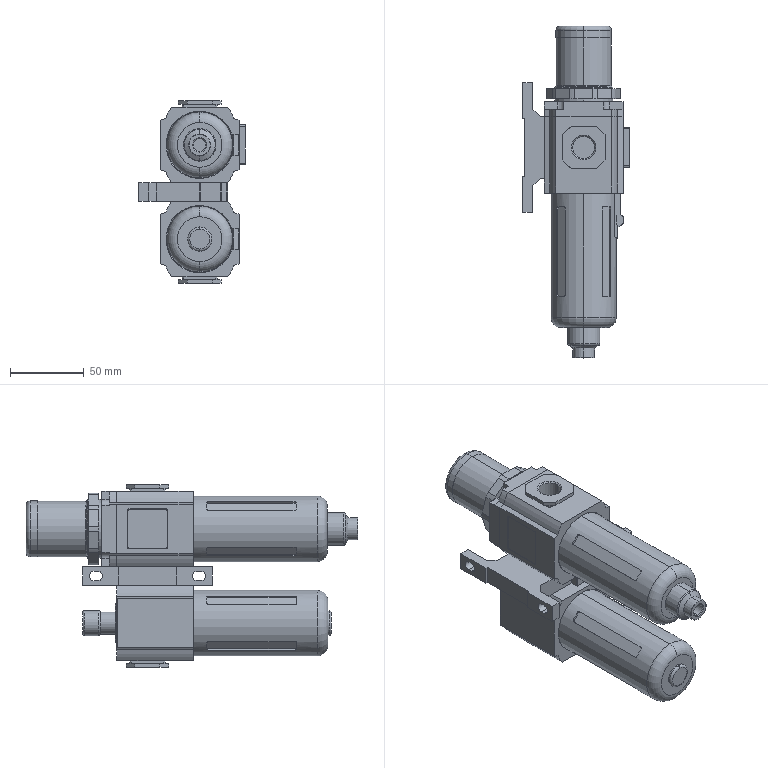Part | SolidWorks | features AEMSimFeature 1 | 9 solids | 584 faces | box 72.5 x 225.5 x 124 mm | volume 471069 mm3 | plane 336 | cylinder 190 | cone 32 | torus 26 | commonest cylinder face diameters 2 x44 4 x22 40 x20 50 x10 14.95 x8 43 x8